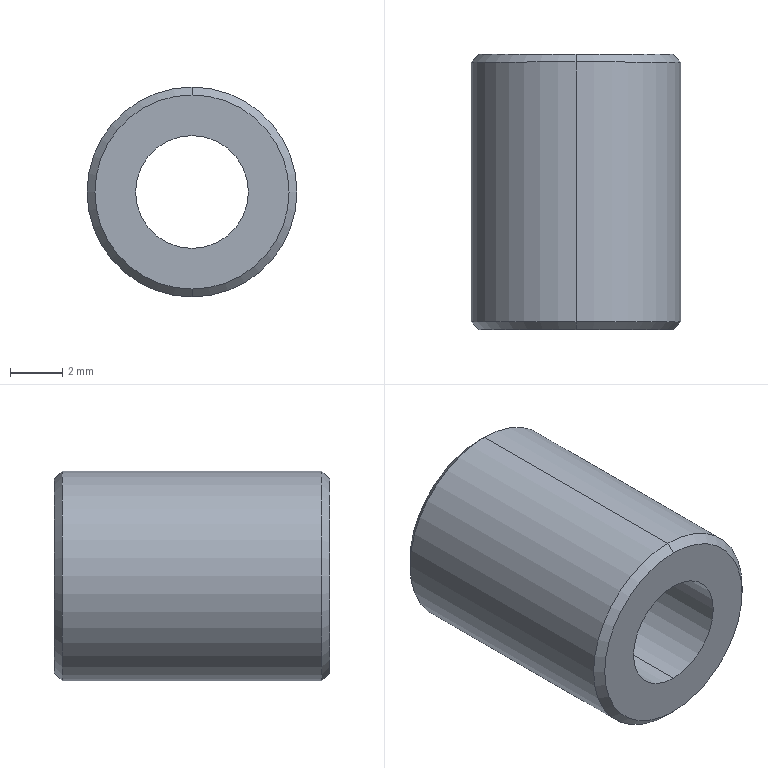Part | STEP file | PN_0004 | 1 solid | 10 faces | box 8 x 10.5 x 8 mm | volume 373.101 mm3 | cone 4 | cylinder 4 | plane 2 | commonest cylinder face diameters 4.3 x2 8 x2
STEP:
#1=CARTESIAN_POINT('',(0.,0.,0.));
#2=DIRECTION('',(0.,0.,1.));
#3=DIRECTION('',(1.,0.,0.));
#4=AXIS2_PLACEMENT_3D('',#1,#2,#3);
#5=CARTESIAN_POINT('',(0.,5.25,3.7));
#6=VERTEX_POINT('',#5);
#7=CARTESIAN_POINT('',(0.,5.25,-3.7));
#8=VERTEX_POINT('',#7);
#9=CARTESIAN_POINT('',(0.,5.25,0.));
#10=DIRECTION('',(0.,1.,0.));
#11=DIRECTION('',(0.,0.,1.));
#12=AXIS2_PLACEMENT_3D('',#9,#10,#11);
#13=CIRCLE('',#12,3.7);
#14=CARTESIAN_POINT('',(0.,5.25,0.));
#15=DIRECTION('',(0.,-1.,0.));
#16=DIRECTION('',(0.,0.,-1.));
#17=AXIS2_PLACEMENT_3D('',#14,#15,#16);
#18=CONICAL_SURFACE('',#17,3.7,0.7854);
#19=CARTESIAN_POINT('',(3.142,0.));
#20=DIRECTION('',(-1.,0.));
#21=VECTOR('',#20,1.);
#22=LINE('',#19,#21);
#23=(GEOMETRIC_REPRESENTATION_CONTEXT(2)PARAMETRIC_REPRESENTATION_CONTEXT()REPRESENTATION_CONTEXT('',''));
#24=DEFINITIONAL_REPRESENTATION('',(#22),#23);
#25=PCURVE('',#18,#24);
#26=CARTESIAN_POINT('',(0.,5.25,0.));
#27=DIRECTION('',(0.,1.,0.));
#28=DIRECTION('',(0.,0.,1.));
#29=AXIS2_PLACEMENT_3D('',#26,#27,#28);
#30=PLANE('',#29);
#31=CARTESIAN_POINT('',(0.,0.));
#32=DIRECTION('',(1.,0.));
#33=AXIS2_PLACEMENT_2D('',#31,#32);
#34=CIRCLE('',#33,3.7);
#35=(GEOMETRIC_REPRESENTATION_CONTEXT(2)PARAMETRIC_REPRESENTATION_CONTEXT()REPRESENTATION_CONTEXT('',''));
#36=DEFINITIONAL_REPRESENTATION('',(#34),#35);
#37=PCURVE('',#30,#36);
#38=SURFACE_CURVE('',#13,(#25,#37),.PCURVE_S1.);
#39=EDGE_CURVE('',#6,#8,#38,.T.);
#40=ORIENTED_EDGE('',*,*,#39,.F.);
#41=CARTESIAN_POINT('',(0.,4.95,4.));
#42=VERTEX_POINT('',#41);
#43=CARTESIAN_POINT('',(0.,5.25,3.7));
#44=DIRECTION('',(0.,-0.7071,0.7071));
#45=VECTOR('',#44,1.);
#46=LINE('',#43,#45);
#47=CARTESIAN_POINT('',(3.142,0.));
#48=DIRECTION('',(0.,1.));
#49=VECTOR('',#48,1.);
#50=LINE('',#47,#49);
#51=(GEOMETRIC_REPRESENTATION_CONTEXT(2)PARAMETRIC_REPRESENTATION_CONTEXT()REPRESENTATION_CONTEXT('',''));
#52=DEFINITIONAL_REPRESENTATION('',(#50),#51);
#53=PCURVE('',#18,#52);
#54=CARTESIAN_POINT('',(0.,5.25,0.));
#55=DIRECTION('',(0.,-1.,0.));
#56=DIRECTION('',(0.,0.,-1.));
#57=AXIS2_PLACEMENT_3D('',#54,#55,#56);
#58=CONICAL_SURFACE('',#57,3.7,0.7854);
#59=CARTESIAN_POINT('',(3.142,0.));
#60=DIRECTION('',(0.,1.));
#61=VECTOR('',#60,1.);
#62=LINE('',#59,#61);
#63=(GEOMETRIC_REPRESENTATION_CONTEXT(2)PARAMETRIC_REPRESENTATION_CONTEXT()REPRESENTATION_CONTEXT('',''));
#64=DEFINITIONAL_REPRESENTATION('',(#62),#63);
#65=PCURVE('',#58,#64);
#66=SURFACE_CURVE('',#46,(#53,#65),.PCURVE_S1.);
#67=EDGE_CURVE('',#6,#42,#66,.T.);
#68=ORIENTED_EDGE('',*,*,#67,.T.);
#69=CARTESIAN_POINT('',(0.,4.95,-4.));
#70=VERTEX_POINT('',#69);
#71=CARTESIAN_POINT('',(0.,4.95,0.));
#72=DIRECTION('',(0.,-1.,0.));
#73=DIRECTION('',(0.,0.,1.));
#74=AXIS2_PLACEMENT_3D('',#71,#72,#73);
#75=CIRCLE('',#74,4.);
#76=CARTESIAN_POINT('',(-3.142,0.3));
#77=DIRECTION('',(1.,0.));
#78=VECTOR('',#77,1.);
#79=LINE('',#76,#78);
#80=(GEOMETRIC_REPRESENTATION_CONTEXT(2)PARAMETRIC_REPRESENTATION_CONTEXT()REPRESENTATION_CONTEXT('',''));
#81=DEFINITIONAL_REPRESENTATION('',(#79),#80);
#82=PCURVE('',#18,#81);
#83=CARTESIAN_POINT('',(0.,5.25,0.));
#84=DIRECTION('',(0.,-1.,0.));
#85=DIRECTION('',(0.,0.,-1.));
#86=AXIS2_PLACEMENT_3D('',#83,#84,#85);
#87=CYLINDRICAL_SURFACE('',#86,4.);
#88=CARTESIAN_POINT('',(-3.142,0.3));
#89=DIRECTION('',(1.,0.));
#90=VECTOR('',#89,1.);
#91=LINE('',#88,#90);
#92=(GEOMETRIC_REPRESENTATION_CONTEXT(2)PARAMETRIC_REPRESENTATION_CONTEXT()REPRESENTATION_CONTEXT('',''));
#93=DEFINITIONAL_REPRESENTATION('',(#91),#92);
#94=PCURVE('',#87,#93);
#95=SURFACE_CURVE('',#75,(#82,#94),.PCURVE_S1.);
#96=EDGE_CURVE('',#70,#42,#95,.T.);
#97=ORIENTED_EDGE('',*,*,#96,.F.);
#98=CARTESIAN_POINT('',(0.,5.25,-3.7));
#99=DIRECTION('',(0.,-0.7071,-0.7071));
#100=VECTOR('',#99,1.);
#101=LINE('',#98,#100);
#102=CARTESIAN_POINT('',(0.,0.));
#103=DIRECTION('',(0.,1.));
#104=VECTOR('',#103,1.);
#105=LINE('',#102,#104);
#106=(GEOMETRIC_REPRESENTATION_CONTEXT(2)PARAMETRIC_REPRESENTATION_CONTEXT()REPRESENTATION_CONTEXT('',''));
#107=DEFINITIONAL_REPRESENTATION('',(#105),#106);
#108=PCURVE('',#18,#107);
#109=CARTESIAN_POINT('',(6.283,0.));
#110=DIRECTION('',(0.,1.));
#111=VECTOR('',#110,1.);
#112=LINE('',#109,#111);
#113=(GEOMETRIC_REPRESENTATION_CONTEXT(2)PARAMETRIC_REPRESENTATION_CONTEXT()REPRESENTATION_CONTEXT('',''));
#114=DEFINITIONAL_REPRESENTATION('',(#112),#113);
#115=PCURVE('',#58,#114);
#116=SURFACE_CURVE('',#101,(#108,#115),.PCURVE_S1.);
#117=EDGE_CURVE('',#8,#70,#116,.T.);
#118=ORIENTED_EDGE('',*,*,#117,.F.);
#119=EDGE_LOOP('',(#40,#68,#97,#118));
#120=FACE_BOUND('',#119,.T.);
#121=ADVANCED_FACE('',(#120),#18,.T.);
#122=CARTESIAN_POINT('',(0.,-5.25,-3.7));
#123=VERTEX_POINT('',#122);
#124=CARTESIAN_POINT('',(0.,-5.25,3.7));
#125=VERTEX_POINT('',#124);
#126=CARTESIAN_POINT('',(0.,-5.25,0.));
#127=DIRECTION('',(0.,-1.,0.));
#128=DIRECTION('',(0.,0.,1.));
#129=AXIS2_PLACEMENT_3D('',#126,#127,#128);
#130=CIRCLE('',#129,3.7);
#131=CARTESIAN_POINT('',(0.,-4.95,0.));
#132=DIRECTION('',(0.,1.,0.));
#133=DIRECTION('',(0.,0.,1.));
#134=AXIS2_PLACEMENT_3D('',#131,#132,#133);
#135=CONICAL_SURFACE('',#134,4.,0.7854);
#136=CARTESIAN_POINT('',(6.283,-0.3));
#137=DIRECTION('',(-1.,0.));
#138=VECTOR('',#137,1.);
#139=LINE('',#136,#138);
#140=(GEOMETRIC_REPRESENTATION_CONTEXT(2)PARAMETRIC_REPRESENTATION_CONTEXT()REPRESENTATION_CONTEXT('',''));
#141=DEFINITIONAL_REPRESENTATION('',(#139),#140);
#142=PCURVE('',#135,#141);
#143=CARTESIAN_POINT('',(0.,-5.25,0.));
#144=DIRECTION('',(0.,1.,0.));
#145=DIRECTION('',(0.,0.,1.));
#146=AXIS2_PLACEMENT_3D('',#143,#144,#145);
#147=PLANE('',#146);
#148=CARTESIAN_POINT('',(3.7,0.));
#149=CARTESIAN_POINT('',(3.7,-6.409));
#150=CARTESIAN_POINT('',(-1.85,-3.204));
#151=CARTESIAN_POINT('',(-7.4,0.));
#152=CARTESIAN_POINT('',(-1.85,3.204));
#153=CARTESIAN_POINT('',(3.7,6.409));
#154=CARTESIAN_POINT('',(3.7,0.));
#155=(BOUNDED_CURVE()B_SPLINE_CURVE(2,(#148,#149,#150,#151,#152,#153,#154),.UNSPECIFIED.,.T.,.F.)B_SPLINE_CURVE_WITH_KNOTS((1,2,2,2,2,1),(-2.094,0.,2.094,4.189,6.283,8.378),.UNSPECIFIED.)CURVE()GEOMETRIC_REPRESENTATION_ITEM()RATIONAL_B_SPLINE_CURVE((1.,0.5,1.,0.5,1.,0.5,1.))REPRESENTATION_ITEM(''));
#156=(GEOMETRIC_REPRESENTATION_CONTEXT(2)PARAMETRIC_REPRESENTATION_CONTEXT()REPRESENTATION_CONTEXT('',''));
#157=DEFINITIONAL_REPRESENTATION('',(#155),#156);
#158=PCURVE('',#147,#157);
#159=SURFACE_CURVE('',#130,(#142,#158),.PCURVE_S1.);
#160=EDGE_CURVE('',#123,#125,#159,.T.);
#161=ORIENTED_EDGE('',*,*,#160,.F.);
#162=CARTESIAN_POINT('',(0.,-4.95,-4.));
#163=VERTEX_POINT('',#162);
#164=CARTESIAN_POINT('',(0.,-4.95,-4.));
#165=DIRECTION('',(0.,0.7071,-0.7071));
#166=VECTOR('',#165,1.);
#167=LINE('',#164,#166);
#168=CARTESIAN_POINT('',(3.142,0.));
#169=DIRECTION('',(0.,1.));
#170=VECTOR('',#169,1.);
#171=LINE('',#168,#170);
#172=(GEOMETRIC_REPRESENTATION_CONTEXT(2)PARAMETRIC_REPRESENTATION_CONTEXT()REPRESENTATION_CONTEXT('',''));
#173=DEFINITIONAL_REPRESENTATION('',(#171),#172);
#174=PCURVE('',#135,#173);
#175=CARTESIAN_POINT('',(0.,-4.95,0.));
#176=DIRECTION('',(0.,1.,0.));
#177=DIRECTION('',(0.,0.,1.));
#178=AXIS2_PLACEMENT_3D('',#175,#176,#177);
#179=CONICAL_SURFACE('',#178,4.,0.7854);
#180=CARTESIAN_POINT('',(3.142,0.));
#181=DIRECTION('',(0.,1.));
#182=VECTOR('',#181,1.);
#183=LINE('',#180,#182);
#184=(GEOMETRIC_REPRESENTATION_CONTEXT(2)PARAMETRIC_REPRESENTATION_CONTEXT()REPRESENTATION_CONTEXT('',''));
#185=DEFINITIONAL_REPRESENTATION('',(#183),#184);
#186=PCURVE('',#179,#185);
#187=SURFACE_CURVE('',#167,(#174,#186),.PCURVE_S1.);
#188=EDGE_CURVE('',#123,#163,#187,.T.);
#189=ORIENTED_EDGE('',*,*,#188,.T.);
#190=CARTESIAN_POINT('',(0.,-4.95,4.));
#191=VERTEX_POINT('',#190);
#192=CARTESIAN_POINT('',(0.,-4.95,0.));
#193=DIRECTION('',(0.,1.,0.));
#194=DIRECTION('',(0.,0.,1.));
#195=AXIS2_PLACEMENT_3D('',#192,#193,#194);
#196=CIRCLE('',#195,4.);
#197=CARTESIAN_POINT('',(0.,0.));
#198=DIRECTION('',(1.,0.));
#199=VECTOR('',#198,1.);
#200=LINE('',#197,#199);
#201=(GEOMETRIC_REPRESENTATION_CONTEXT(2)PARAMETRIC_REPRESENTATION_CONTEXT()REPRESENTATION_CONTEXT('',''));
#202=DEFINITIONAL_REPRESENTATION('',(#200),#201);
#203=PCURVE('',#135,#202);
#204=CARTESIAN_POINT('',(3.142,10.2));
#205=DIRECTION('',(-1.,0.));
#206=VECTOR('',#205,1.);
#207=LINE('',#204,#206);
#208=(GEOMETRIC_REPRESENTATION_CONTEXT(2)PARAMETRIC_REPRESENTATION_CONTEXT()REPRESENTATION_CONTEXT('',''));
#209=DEFINITIONAL_REPRESENTATION('',(#207),#208);
#210=PCURVE('',#87,#209);
#211=SURFACE_CURVE('',#196,(#203,#210),.PCURVE_S1.);
#212=EDGE_CURVE('',#191,#163,#211,.T.);
#213=ORIENTED_EDGE('',*,*,#212,.F.);
#214=CARTESIAN_POINT('',(0.,-4.95,4.));
#215=DIRECTION('',(0.,0.7071,0.7071));
#216=VECTOR('',#215,1.);
#217=LINE('',#214,#216);
#218=CARTESIAN_POINT('',(0.,0.));
#219=DIRECTION('',(0.,1.));
#220=VECTOR('',#219,1.);
#221=LINE('',#218,#220);
#222=(GEOMETRIC_REPRESENTATION_CONTEXT(2)PARAMETRIC_REPRESENTATION_CONTEXT()REPRESENTATION_CONTEXT('',''));
#223=DEFINITIONAL_REPRESENTATION('',(#221),#222);
#224=PCURVE('',#135,#223);
#225=CARTESIAN_POINT('',(6.283,0.));
#226=DIRECTION('',(0.,1.));
#227=VECTOR('',#226,1.);
#228=LINE('',#225,#227);
#229=(GEOMETRIC_REPRESENTATION_CONTEXT(2)PARAMETRIC_REPRESENTATION_CONTEXT()REPRESENTATION_CONTEXT('',''));
#230=DEFINITIONAL_REPRESENTATION('',(#228),#229);
#231=PCURVE('',#179,#230);
#232=SURFACE_CURVE('',#217,(#224,#231),.PCURVE_S1.);
#233=EDGE_CURVE('',#125,#191,#232,.T.);
#234=ORIENTED_EDGE('',*,*,#233,.F.);
#235=EDGE_LOOP('',(#161,#189,#213,#234));
#236=FACE_BOUND('',#235,.T.);
#237=ADVANCED_FACE('',(#236),#135,.T.);
#238=CARTESIAN_POINT('',(0.,5.25,-2.15));
#239=VERTEX_POINT('',#238);
#240=CARTESIAN_POINT('',(0.,-5.25,-2.15));
#241=VERTEX_POINT('',#240);
#242=CARTESIAN_POINT('',(0.,-5.25,-2.15));
#243=DIRECTION('',(0.,-1.,0.));
#244=VECTOR('',#243,1.);
#245=LINE('',#242,#244);
#246=CARTESIAN_POINT('',(0.,-5.25,0.));
#247=DIRECTION('',(0.,-1.,0.));
#248=DIRECTION('',(0.,0.,-1.));
#249=AXIS2_PLACEMENT_3D('',#246,#247,#248);
#250=CYLINDRICAL_SURFACE('',#249,2.15);
#251=CARTESIAN_POINT('',(6.283,0.));
#252=DIRECTION('',(0.,1.));
#253=VECTOR('',#252,1.);
#254=LINE('',#251,#253);
#255=(GEOMETRIC_REPRESENTATION_CONTEXT(2)PARAMETRIC_REPRESENTATION_CONTEXT()REPRESENTATION_CONTEXT('',''));
#256=DEFINITIONAL_REPRESENTATION('',(#254),#255);
#257=PCURVE('',#250,#256);
#258=CARTESIAN_POINT('',(0.,-5.25,0.));
#259=DIRECTION('',(0.,-1.,0.));
#260=DIRECTION('',(0.,0.,-1.));
#261=AXIS2_PLACEMENT_3D('',#258,#259,#260);
#262=CYLINDRICAL_SURFACE('',#261,2.15);
#263=CARTESIAN_POINT('',(0.,0.));
#264=DIRECTION('',(0.,1.));
#265=VECTOR('',#264,1.);
#266=LINE('',#263,#265);
#267=(GEOMETRIC_REPRESENTATION_CONTEXT(2)PARAMETRIC_REPRESENTATION_CONTEXT()REPRESENTATION_CONTEXT('',''));
#268=DEFINITIONAL_REPRESENTATION('',(#266),#267);
#269=PCURVE('',#262,#268);
#270=SURFACE_CURVE('',#245,(#257,#269),.PCURVE_S1.);
#271=EDGE_CURVE('',#239,#241,#270,.T.);
#272=ORIENTED_EDGE('',*,*,#271,.T.);
#273=CARTESIAN_POINT('',(0.,-5.25,2.15));
#274=VERTEX_POINT('',#273);
#275=CARTESIAN_POINT('',(0.,-5.25,0.));
#276=DIRECTION('',(0.,-1.,0.));
#277=DIRECTION('',(0.,0.,-1.));
#278=AXIS2_PLACEMENT_3D('',#275,#276,#277);
#279=CIRCLE('',#278,2.15);
#280=CARTESIAN_POINT('',(0.,0.));
#281=DIRECTION('',(1.,0.));
#282=VECTOR('',#281,1.);
#283=LINE('',#280,#282);
#284=(GEOMETRIC_REPRESENTATION_CONTEXT(2)PARAMETRIC_REPRESENTATION_CONTEXT()REPRESENTATION_CONTEXT('',''));
#285=DEFINITIONAL_REPRESENTATION('',(#283),#284);
#286=PCURVE('',#250,#285);
#287=CARTESIAN_POINT('',(-2.15,0.));
#288=CARTESIAN_POINT('',(-2.15,3.724));
#289=CARTESIAN_POINT('',(1.075,1.862));
#290=CARTESIAN_POINT('',(4.3,0.));
#291=CARTESIAN_POINT('',(1.075,-1.862));
#292=CARTESIAN_POINT('',(-2.15,-3.724));
#293=CARTESIAN_POINT('',(-2.15,0.));
#294=(BOUNDED_CURVE()B_SPLINE_CURVE(2,(#287,#288,#289,#290,#291,#292,#293),.UNSPECIFIED.,.T.,.F.)B_SPLINE_CURVE_WITH_KNOTS((1,2,2,2,2,1),(-2.094,0.,2.094,4.189,6.283,8.378),.UNSPECIFIED.)CURVE()GEOMETRIC_REPRESENTATION_ITEM()RATIONAL_B_SPLINE_CURVE((1.,0.5,1.,0.5,1.,0.5,1.))REPRESENTATION_ITEM(''));
#295=(GEOMETRIC_REPRESENTATION_CONTEXT(2)PARAMETRIC_REPRESENTATION_CONTEXT()REPRESENTATION_CONTEXT('',''));
#296=DEFINITIONAL_REPRESENTATION('',(#294),#295);
#297=PCURVE('',#147,#296);
#298=SURFACE_CURVE('',#279,(#286,#297),.PCURVE_S1.);
#299=EDGE_CURVE('',#274,#241,#298,.T.);
#300=ORIENTED_EDGE('',*,*,#299,.F.);
#301=CARTESIAN_POINT('',(0.,5.25,2.15));
#302=VERTEX_POINT('',#301);
#303=CARTESIAN_POINT('',(0.,-5.25,2.15));
#304=DIRECTION('',(0.,-1.,0.));
#305=VECTOR('',#304,1.);
#306=LINE('',#303,#305);
#307=CARTESIAN_POINT('',(3.142,0.));
#308=DIRECTION('',(0.,1.));
#309=VECTOR('',#308,1.);
#310=LINE('',#307,#309);
#311=(GEOMETRIC_REPRESENTATION_CONTEXT(2)PARAMETRIC_REPRESENTATION_CONTEXT()REPRESENTATION_CONTEXT('',''));
#312=DEFINITIONAL_REPRESENTATION('',(#310),#311);
#313=PCURVE('',#250,#312);
#314=CARTESIAN_POINT('',(3.142,0.));
#315=DIRECTION('',(0.,1.));
#316=VECTOR('',#315,1.);
#317=LINE('',#314,#316);
#318=(GEOMETRIC_REPRESENTATION_CONTEXT(2)PARAMETRIC_REPRESENTATION_CONTEXT()REPRESENTATION_CONTEXT('',''));
#319=DEFINITIONAL_REPRESENTATION('',(#317),#318);
#320=PCURVE('',#262,#319);
#321=SURFACE_CURVE('',#306,(#313,#320),.PCURVE_S1.);
#322=EDGE_CURVE('',#302,#274,#321,.T.);
#323=ORIENTED_EDGE('',*,*,#322,.F.);
#324=CARTESIAN_POINT('',(0.,5.25,0.));
#325=DIRECTION('',(0.,-1.,0.));
#326=DIRECTION('',(0.,0.,-1.));
#327=AXIS2_PLACEMENT_3D('',#324,#325,#326);
#328=CIRCLE('',#327,2.15);
#329=CARTESIAN_POINT('',(0.,-10.5));
#330=DIRECTION('',(1.,0.));
#331=VECTOR('',#330,1.);
#332=LINE('',#329,#331);
#333=(GEOMETRIC_REPRESENTATION_CONTEXT(2)PARAMETRIC_REPRESENTATION_CONTEXT()REPRESENTATION_CONTEXT('',''));
#334=DEFINITIONAL_REPRESENTATION('',(#332),#333);
#335=PCURVE('',#250,#334);
#336=CARTESIAN_POINT('',(-2.15,0.));
#337=CARTESIAN_POINT('',(-2.15,3.724));
#338=CARTESIAN_POINT('',(1.075,1.862));
#339=CARTESIAN_POINT('',(4.3,0.));
#340=CARTESIAN_POINT('',(1.075,-1.862));
#341=CARTESIAN_POINT('',(-2.15,-3.724));
#342=CARTESIAN_POINT('',(-2.15,0.));
#343=(BOUNDED_CURVE()B_SPLINE_CURVE(2,(#336,#337,#338,#339,#340,#341,#342),.UNSPECIFIED.,.T.,.F.)B_SPLINE_CURVE_WITH_KNOTS((1,2,2,2,2,1),(-2.094,0.,2.094,4.189,6.283,8.378),.UNSPECIFIED.)CURVE()GEOMETRIC_REPRESENTATION_ITEM()RATIONAL_B_SPLINE_CURVE((1.,0.5,1.,0.5,1.,0.5,1.))REPRESENTATION_ITEM(''));
#344=(GEOMETRIC_REPRESENTATION_CONTEXT(2)PARAMETRIC_REPRESENTATION_CONTEXT()REPRESENTATION_CONTEXT('',''));
#345=DEFINITIONAL_REPRESENTATION('',(#343),#344);
#346=PCURVE('',#30,#345);
#347=SURFACE_CURVE('',#328,(#335,#346),.PCURVE_S1.);
#348=EDGE_CURVE('',#302,#239,#347,.T.);
#349=ORIENTED_EDGE('',*,*,#348,.T.);
#350=EDGE_LOOP('',(#272,#300,#323,#349));
#351=FACE_BOUND('',#350,.F.);
#352=ADVANCED_FACE('',(#351),#250,.F.);
#353=ORIENTED_EDGE('',*,*,#96,.T.);
#354=CARTESIAN_POINT('',(0.,5.25,4.));
#355=DIRECTION('',(0.,-1.,0.));
#356=VECTOR('',#355,1.);
#357=LINE('',#354,#356);
#358=CARTESIAN_POINT('',(3.142,0.));
#359=DIRECTION('',(0.,1.));
#360=VECTOR('',#359,1.);
#361=LINE('',#358,#360);
#362=(GEOMETRIC_REPRESENTATION_CONTEXT(2)PARAMETRIC_REPRESENTATION_CONTEXT()REPRESENTATION_CONTEXT('',''));
#363=DEFINITIONAL_REPRESENTATION('',(#361),#362);
#364=PCURVE('',#87,#363);
#365=CARTESIAN_POINT('',(0.,5.25,0.));
#366=DIRECTION('',(0.,-1.,0.));
#367=DIRECTION('',(0.,0.,-1.));
#368=AXIS2_PLACEMENT_3D('',#365,#366,#367);
#369=CYLINDRICAL_SURFACE('',#368,4.);
#370=CARTESIAN_POINT('',(3.142,0.));
#371=DIRECTION('',(0.,1.));
#372=VECTOR('',#371,1.);
#373=LINE('',#370,#372);
#374=(GEOMETRIC_REPRESENTATION_CONTEXT(2)PARAMETRIC_REPRESENTATION_CONTEXT()REPRESENTATION_CONTEXT('',''));
#375=DEFINITIONAL_REPRESENTATION('',(#373),#374);
#376=PCURVE('',#369,#375);
#377=SURFACE_CURVE('',#357,(#364,#376),.PCURVE_S1.);
#378=EDGE_CURVE('',#42,#191,#377,.T.);
#379=ORIENTED_EDGE('',*,*,#378,.T.);
#380=ORIENTED_EDGE('',*,*,#212,.T.);
#381=CARTESIAN_POINT('',(0.,5.25,-4.));
#382=DIRECTION('',(0.,-1.,0.));
#383=VECTOR('',#382,1.);
#384=LINE('',#381,#383);
#385=CARTESIAN_POINT('',(0.,0.));
#386=DIRECTION('',(0.,1.));
#387=VECTOR('',#386,1.);
#388=LINE('',#385,#387);
#389=(GEOMETRIC_REPRESENTATION_CONTEXT(2)PARAMETRIC_REPRESENTATION_CONTEXT()REPRESENTATION_CONTEXT('',''));
#390=DEFINITIONAL_REPRESENTATION('',(#388),#389);
#391=PCURVE('',#87,#390);
#392=CARTESIAN_POINT('',(6.283,0.));
#393=DIRECTION('',(0.,1.));
#394=VECTOR('',#393,1.);
#395=LINE('',#392,#394);
#396=(GEOMETRIC_REPRESENTATION_CONTEXT(2)PARAMETRIC_REPRESENTATION_CONTEXT()REPRESENTATION_CONTEXT('',''));
#397=DEFINITIONAL_REPRESENTATION('',(#395),#396);
#398=PCURVE('',#369,#397);
#399=SURFACE_CURVE('',#384,(#391,#398),.PCURVE_S1.);
#400=EDGE_CURVE('',#70,#163,#399,.T.);
#401=ORIENTED_EDGE('',*,*,#400,.F.);
#402=EDGE_LOOP('',(#353,#379,#380,#401));
#403=FACE_BOUND('',#402,.T.);
#404=ADVANCED_FACE('',(#403),#87,.T.);
#405=ORIENTED_EDGE('',*,*,#378,.F.);
#406=CARTESIAN_POINT('',(0.,4.95,0.));
#407=DIRECTION('',(0.,-1.,0.));
#408=DIRECTION('',(0.,0.,1.));
#409=AXIS2_PLACEMENT_3D('',#406,#407,#408);
#410=CIRCLE('',#409,4.);
#411=CARTESIAN_POINT('',(3.142,0.3));
#412=DIRECTION('',(1.,0.));
#413=VECTOR('',#412,1.);
#414=LINE('',#411,#413);
#415=(GEOMETRIC_REPRESENTATION_CONTEXT(2)PARAMETRIC_REPRESENTATION_CONTEXT()REPRESENTATION_CONTEXT('',''));
#416=DEFINITIONAL_REPRESENTATION('',(#414),#415);
#417=PCURVE('',#369,#416);
#418=CARTESIAN_POINT('',(3.142,0.3));
#419=DIRECTION('',(1.,0.));
#420=VECTOR('',#419,1.);
#421=LINE('',#418,#420);
#422=(GEOMETRIC_REPRESENTATION_CONTEXT(2)PARAMETRIC_REPRESENTATION_CONTEXT()REPRESENTATION_CONTEXT('',''));
#423=DEFINITIONAL_REPRESENTATION('',(#421),#422);
#424=PCURVE('',#58,#423);
#425=SURFACE_CURVE('',#410,(#417,#424),.PCURVE_S1.);
#426=EDGE_CURVE('',#42,#70,#425,.T.);
#427=ORIENTED_EDGE('',*,*,#426,.T.);
#428=ORIENTED_EDGE('',*,*,#400,.T.);
#429=CARTESIAN_POINT('',(0.,-4.95,0.));
#430=DIRECTION('',(0.,1.,0.));
#431=DIRECTION('',(0.,0.,1.));
#432=AXIS2_PLACEMENT_3D('',#429,#430,#431);
#433=CIRCLE('',#432,4.);
#434=CARTESIAN_POINT('',(9.425,10.2));
#435=DIRECTION('',(-1.,0.));
#436=VECTOR('',#435,1.);
#437=LINE('',#434,#436);
#438=(GEOMETRIC_REPRESENTATION_CONTEXT(2)PARAMETRIC_REPRESENTATION_CONTEXT()REPRESENTATION_CONTEXT('',''));
#439=DEFINITIONAL_REPRESENTATION('',(#437),#438);
#440=PCURVE('',#369,#439);
#441=CARTESIAN_POINT('',(0.,0.));
#442=DIRECTION('',(1.,0.));
#443=VECTOR('',#442,1.);
#444=LINE('',#441,#443);
#445=(GEOMETRIC_REPRESENTATION_CONTEXT(2)PARAMETRIC_REPRESENTATION_CONTEXT()REPRESENTATION_CONTEXT('',''));
#446=DEFINITIONAL_REPRESENTATION('',(#444),#445);
#447=PCURVE('',#179,#446);
#448=SURFACE_CURVE('',#433,(#440,#447),.PCURVE_S1.);
#449=EDGE_CURVE('',#163,#191,#448,.T.);
#450=ORIENTED_EDGE('',*,*,#449,.T.);
#451=EDGE_LOOP('',(#405,#427,#428,#450));
#452=FACE_BOUND('',#451,.T.);
#453=ADVANCED_FACE('',(#452),#369,.T.);
#454=CARTESIAN_POINT('',(0.,5.25,0.));
#455=DIRECTION('',(0.,1.,0.));
#456=DIRECTION('',(0.,0.,1.));
#457=AXIS2_PLACEMENT_3D('',#454,#455,#456);
#458=CIRCLE('',#457,3.7);
#459=CARTESIAN_POINT('',(0.,0.));
#460=DIRECTION('',(1.,0.));
#461=AXIS2_PLACEMENT_2D('',#459,#460);
#462=CIRCLE('',#461,3.7);
#463=(GEOMETRIC_REPRESENTATION_CONTEXT(2)PARAMETRIC_REPRESENTATION_CONTEXT()REPRESENTATION_CONTEXT('',''));
#464=DEFINITIONAL_REPRESENTATION('',(#462),#463);
#465=PCURVE('',#30,#464);
#466=CARTESIAN_POINT('',(9.425,0.));
#467=DIRECTION('',(-1.,0.));
#468=VECTOR('',#467,1.);
#469=LINE('',#466,#468);
#470=(GEOMETRIC_REPRESENTATION_CONTEXT(2)PARAMETRIC_REPRESENTATION_CONTEXT()REPRESENTATION_CONTEXT('',''));
#471=DEFINITIONAL_REPRESENTATION('',(#469),#470);
#472=PCURVE('',#58,#471);
#473=SURFACE_CURVE('',#458,(#465,#472),.PCURVE_S1.);
#474=EDGE_CURVE('',#8,#6,#473,.T.);
#475=ORIENTED_EDGE('',*,*,#474,.T.);
#476=ORIENTED_EDGE('',*,*,#39,.T.);
#477=EDGE_LOOP('',(#475,#476));
#478=FACE_BOUND('',#477,.T.);
#479=CARTESIAN_POINT('',(0.,5.25,0.));
#480=DIRECTION('',(0.,-1.,0.));
#481=DIRECTION('',(0.,0.,-1.));
#482=AXIS2_PLACEMENT_3D('',#479,#480,#481);
#483=CIRCLE('',#482,2.15);
#484=CARTESIAN_POINT('',(-2.15,0.));
#485=CARTESIAN_POINT('',(-2.15,3.724));
#486=CARTESIAN_POINT('',(1.075,1.862));
#487=CARTESIAN_POINT('',(4.3,0.));
#488=CARTESIAN_POINT('',(1.075,-1.862));
#489=CARTESIAN_POINT('',(-2.15,-3.724));
#490=CARTESIAN_POINT('',(-2.15,0.));
#491=(BOUNDED_CURVE()B_SPLINE_CURVE(2,(#484,#485,#486,#487,#488,#489,#490),.UNSPECIFIED.,.T.,.F.)B_SPLINE_CURVE_WITH_KNOTS((1,2,2,2,2,1),(-2.094,0.,2.094,4.189,6.283,8.378),.UNSPECIFIED.)CURVE()GEOMETRIC_REPRESENTATION_ITEM()RATIONAL_B_SPLINE_CURVE((1.,0.5,1.,0.5,1.,0.5,1.))REPRESENTATION_ITEM(''));
#492=(GEOMETRIC_REPRESENTATION_CONTEXT(2)PARAMETRIC_REPRESENTATION_CONTEXT()REPRESENTATION_CONTEXT('',''));
#493=DEFINITIONAL_REPRESENTATION('',(#491),#492);
#494=PCURVE('',#30,#493);
#495=CARTESIAN_POINT('',(0.,-10.5));
#496=DIRECTION('',(1.,0.));
#497=VECTOR('',#496,1.);
#498=LINE('',#495,#497);
#499=(GEOMETRIC_REPRESENTATION_CONTEXT(2)PARAMETRIC_REPRESENTATION_CONTEXT()REPRESENTATION_CONTEXT('',''));
#500=DEFINITIONAL_REPRESENTATION('',(#498),#499);
#501=PCURVE('',#262,#500);
#502=SURFACE_CURVE('',#483,(#494,#501),.PCURVE_S1.);
#503=EDGE_CURVE('',#239,#302,#502,.T.);
#504=ORIENTED_EDGE('',*,*,#503,.T.);
#505=ORIENTED_EDGE('',*,*,#348,.T.);
#506=EDGE_LOOP('',(#504,#505));
#507=FACE_BOUND('',#506,.T.);
#508=ADVANCED_FACE('',(#478,#507),#30,.T.);
#509=CARTESIAN_POINT('',(0.,-5.25,0.));
#510=DIRECTION('',(0.,-1.,0.));
#511=DIRECTION('',(0.,0.,1.));
#512=AXIS2_PLACEMENT_3D('',#509,#510,#511);
#513=CIRCLE('',#512,3.7);
#514=CARTESIAN_POINT('',(3.7,0.));
#515=CARTESIAN_POINT('',(3.7,-6.409));
#516=CARTESIAN_POINT('',(-1.85,-3.204));
#517=CARTESIAN_POINT('',(-7.4,0.));
#518=CARTESIAN_POINT('',(-1.85,3.204));
#519=CARTESIAN_POINT('',(3.7,6.409));
#520=CARTESIAN_POINT('',(3.7,0.));
#521=(BOUNDED_CURVE()B_SPLINE_CURVE(2,(#514,#515,#516,#517,#518,#519,#520),.UNSPECIFIED.,.T.,.F.)B_SPLINE_CURVE_WITH_KNOTS((1,2,2,2,2,1),(-2.094,0.,2.094,4.189,6.283,8.378),.UNSPECIFIED.)CURVE()GEOMETRIC_REPRESENTATION_ITEM()RATIONAL_B_SPLINE_CURVE((1.,0.5,1.,0.5,1.,0.5,1.))REPRESENTATION_ITEM(''));
#522=(GEOMETRIC_REPRESENTATION_CONTEXT(2)PARAMETRIC_REPRESENTATION_CONTEXT()REPRESENTATION_CONTEXT('',''));
#523=DEFINITIONAL_REPRESENTATION('',(#521),#522);
#524=PCURVE('',#147,#523);
#525=CARTESIAN_POINT('',(6.283,-0.3));
#526=DIRECTION('',(-1.,0.));
#527=VECTOR('',#526,1.);
#528=LINE('',#525,#527);
#529=(GEOMETRIC_REPRESENTATION_CONTEXT(2)PARAMETRIC_REPRESENTATION_CONTEXT()REPRESENTATION_CONTEXT('',''));
#530=DEFINITIONAL_REPRESENTATION('',(#528),#529);
#531=PCURVE('',#179,#530);
#532=SURFACE_CURVE('',#513,(#524,#531),.PCURVE_S1.);
#533=EDGE_CURVE('',#125,#123,#532,.T.);
#534=ORIENTED_EDGE('',*,*,#533,.T.);
#535=ORIENTED_EDGE('',*,*,#160,.T.);
#536=EDGE_LOOP('',(#534,#535));
#537=FACE_BOUND('',#536,.T.);
#538=CARTESIAN_POINT('',(0.,-5.25,0.));
#539=DIRECTION('',(0.,-1.,0.));
#540=DIRECTION('',(0.,0.,-1.));
#541=AXIS2_PLACEMENT_3D('',#538,#539,#540);
#542=CIRCLE('',#541,2.15);
#543=CARTESIAN_POINT('',(-2.15,0.));
#544=CARTESIAN_POINT('',(-2.15,3.724));
#545=CARTESIAN_POINT('',(1.075,1.862));
#546=CARTESIAN_POINT('',(4.3,0.));
#547=CARTESIAN_POINT('',(1.075,-1.862));
#548=CARTESIAN_POINT('',(-2.15,-3.724));
#549=CARTESIAN_POINT('',(-2.15,0.));
#550=(BOUNDED_CURVE()B_SPLINE_CURVE(2,(#543,#544,#545,#546,#547,#548,#549),.UNSPECIFIED.,.T.,.F.)B_SPLINE_CURVE_WITH_KNOTS((1,2,2,2,2,1),(-2.094,0.,2.094,4.189,6.283,8.378),.UNSPECIFIED.)CURVE()GEOMETRIC_REPRESENTATION_ITEM()RATIONAL_B_SPLINE_CURVE((1.,0.5,1.,0.5,1.,0.5,1.))REPRESENTATION_ITEM(''));
#551=(GEOMETRIC_REPRESENTATION_CONTEXT(2)PARAMETRIC_REPRESENTATION_CONTEXT()REPRESENTATION_CONTEXT('',''));
#552=DEFINITIONAL_REPRESENTATION('',(#550),#551);
#553=PCURVE('',#147,#552);
#554=CARTESIAN_POINT('',(0.,0.));
#555=DIRECTION('',(1.,0.));
#556=VECTOR('',#555,1.);
#557=LINE('',#554,#556);
#558=(GEOMETRIC_REPRESENTATION_CONTEXT(2)PARAMETRIC_REPRESENTATION_CONTEXT()REPRESENTATION_CONTEXT('',''));
#559=DEFINITIONAL_REPRESENTATION('',(#557),#558);
#560=PCURVE('',#262,#559);
#561=SURFACE_CURVE('',#542,(#553,#560),.PCURVE_S1.);
#562=EDGE_CURVE('',#241,#274,#561,.T.);
#563=ORIENTED_EDGE('',*,*,#562,.F.);
#564=ORIENTED_EDGE('',*,*,#299,.F.);
#565=EDGE_LOOP('',(#563,#564));
#566=FACE_BOUND('',#565,.T.);
#567=ADVANCED_FACE('',(#537,#566),#147,.F.);
#568=ORIENTED_EDGE('',*,*,#562,.F.);
#569=ORIENTED_EDGE('',*,*,#271,.F.);
#570=ORIENTED_EDGE('',*,*,#503,.T.);
#571=ORIENTED_EDGE('',*,*,#322,.T.);
#572=EDGE_LOOP('',(#568,#569,#570,#571));
#573=FACE_BOUND('',#572,.F.);
#574=ADVANCED_FACE('',(#573),#262,.F.);
#575=ORIENTED_EDGE('',*,*,#188,.F.);
#576=ORIENTED_EDGE('',*,*,#533,.F.);
#577=ORIENTED_EDGE('',*,*,#233,.T.);
#578=ORIENTED_EDGE('',*,*,#449,.F.);
#579=EDGE_LOOP('',(#575,#576,#577,#578));
#580=FACE_BOUND('',#579,.T.);
#581=ADVANCED_FACE('',(#580),#179,.T.);
#582=ORIENTED_EDGE('',*,*,#67,.F.);
#583=ORIENTED_EDGE('',*,*,#474,.F.);
#584=ORIENTED_EDGE('',*,*,#117,.T.);
#585=ORIENTED_EDGE('',*,*,#426,.F.);
#586=EDGE_LOOP('',(#582,#583,#584,#585));
#587=FACE_BOUND('',#586,.T.);
#588=ADVANCED_FACE('',(#587),#58,.T.);
#589=CLOSED_SHELL('',(#121,#237,#352,#404,#453,#508,#567,#574,#581,#588));
#590=MANIFOLD_SOLID_BREP('',#589);
#591=(LENGTH_UNIT()NAMED_UNIT(*)SI_UNIT(.MILLI.,.METRE.));
#592=UNCERTAINTY_MEASURE_WITH_UNIT(LENGTH_MEASURE(0.0000001),#591,'','');
#593=(NAMED_UNIT(*)PLANE_ANGLE_UNIT()SI_UNIT($,.RADIAN.));
#594=(NAMED_UNIT(*)SI_UNIT($,.STERADIAN.)SOLID_ANGLE_UNIT());
#595=(GEOMETRIC_REPRESENTATION_CONTEXT(3)GLOBAL_UNCERTAINTY_ASSIGNED_CONTEXT((#592))GLOBAL_UNIT_ASSIGNED_CONTEXT((#591,#593,#594))REPRESENTATION_CONTEXT('',''));
#596=ADVANCED_BREP_SHAPE_REPRESENTATION('',(#4,#590),#595);